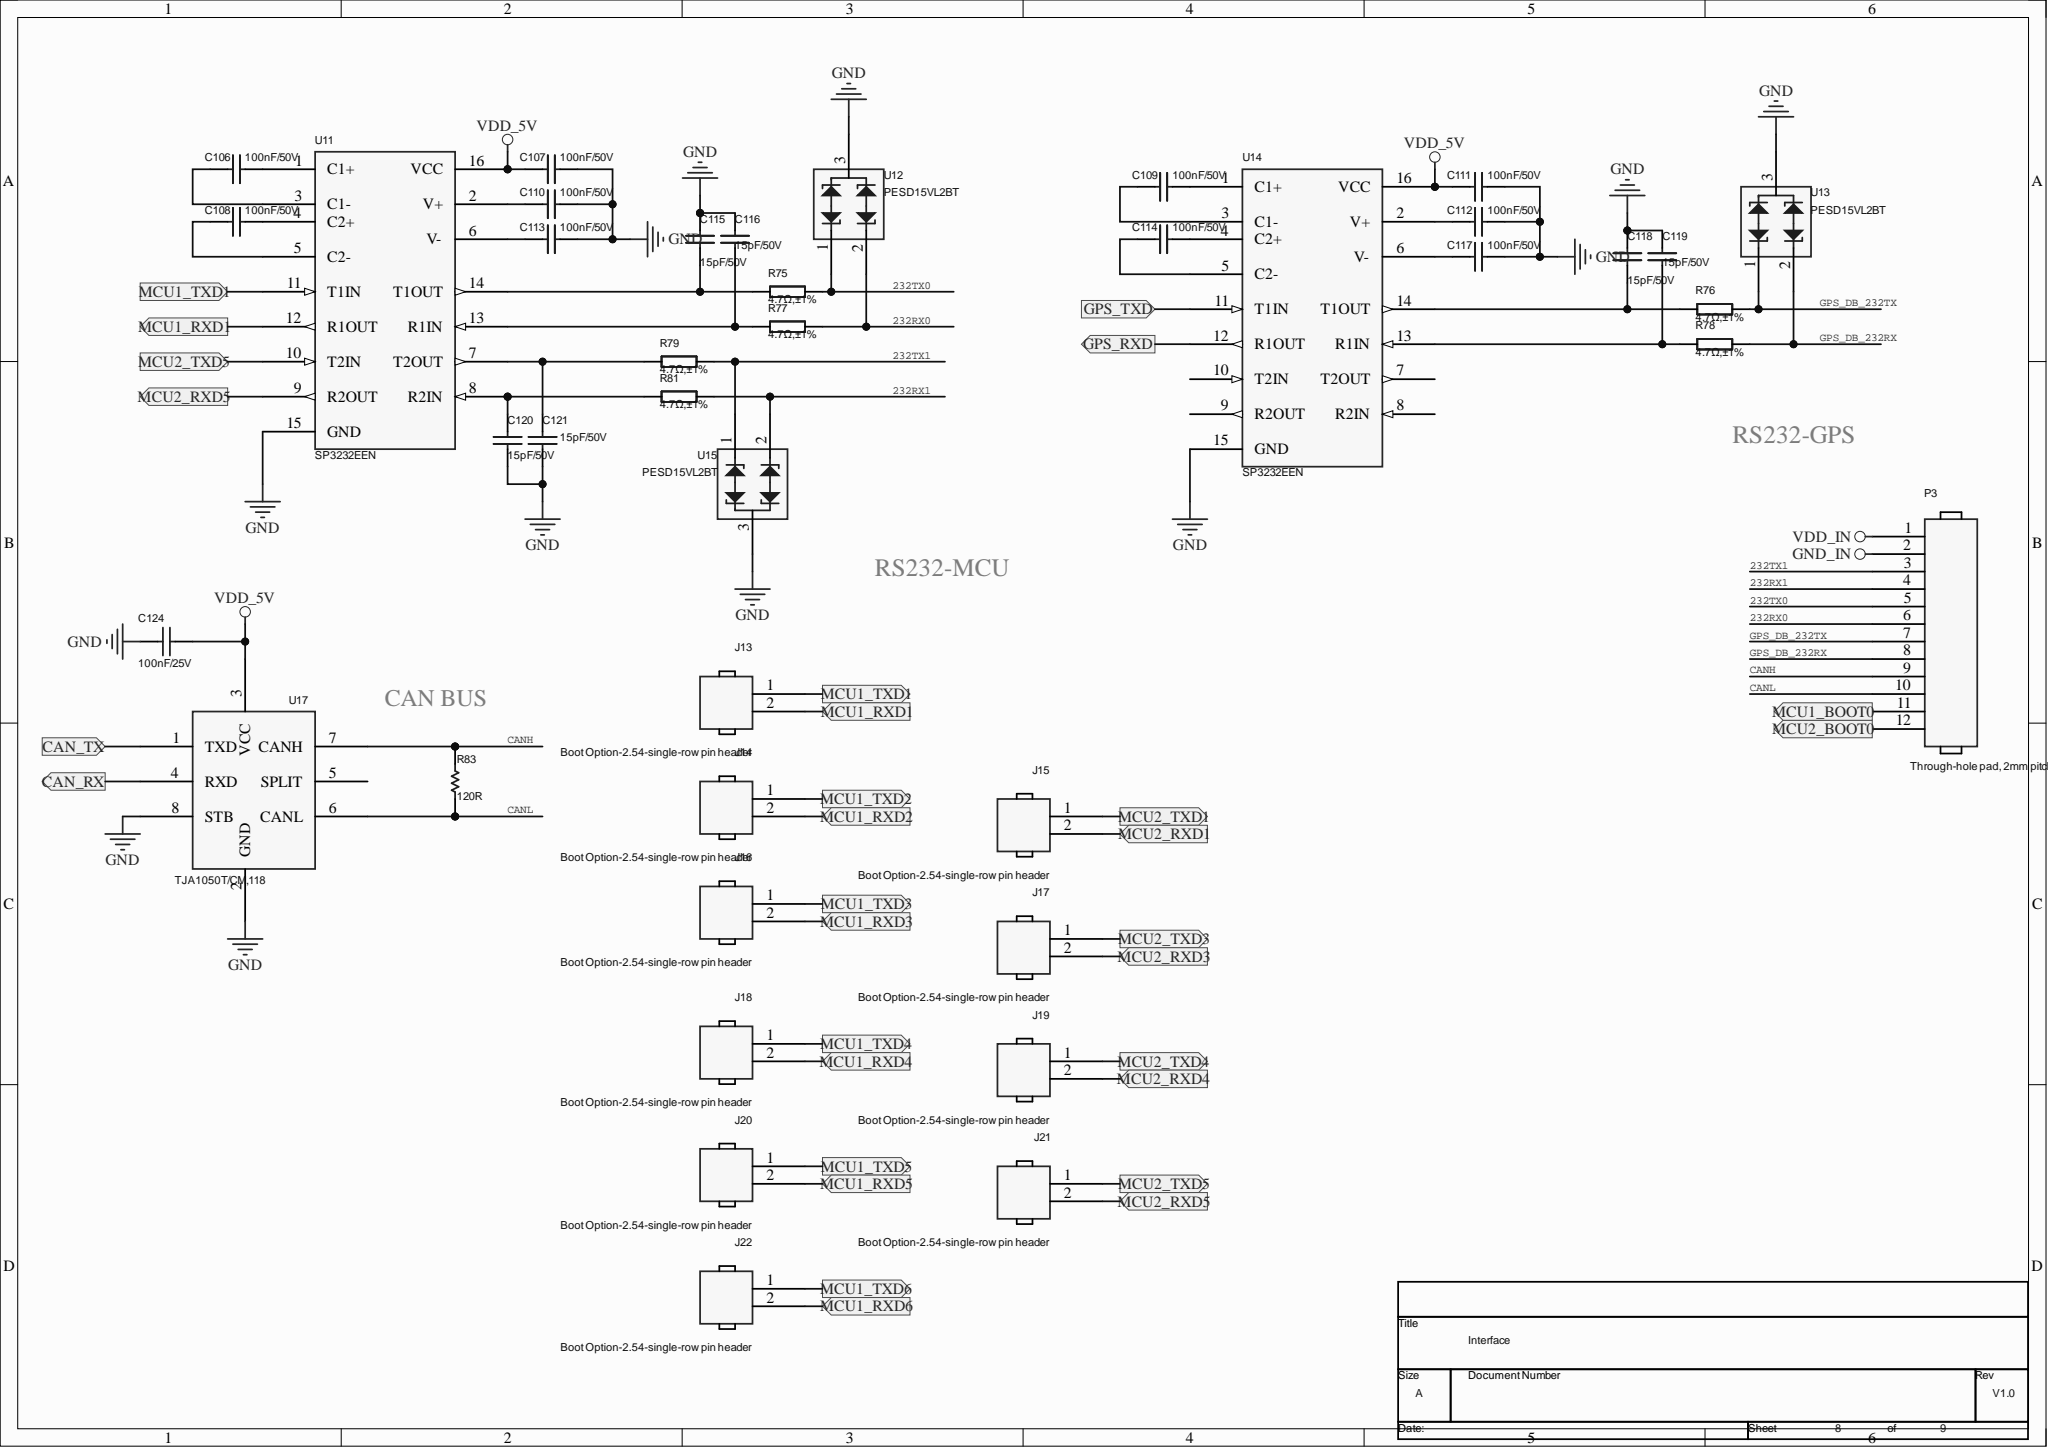Circuit board | Altium Designer | 313 parts | 216 nets | one sheet of the schematic
Parts on this sheet (reference | value | footprint):
C106 | 100nF/50V | 0603
C107 | 100nF/50V | 0603
C108 | 100nF/50V | 0603
C109 | 100nF/50V | 0603
C110 | 100nF/50V | 0603
C111 | 100nF/50V | 0603
C112 | 100nF/50V | 0603
C113 | 100nF/50V | 0603
C114 | 100nF/50V | 0603
C115 | 15pF/50V | 0603
C116 | 15pF/50V | 0603
C117 | 100nF/50V | 0603
C118 | 15pF/50V | 0603
C119 | 15pF/50V | 0603
C120 | 15pF/50V | 0603
C121 | 15pF/50V | 0603
C124 | 100nF/50V | C0603
J13 | Boot Option-2.54-single-row pin header | HDR_1X2_254
J14 | Boot Option-2.54-single-row pin header | HDR_1X2_254
J15 | Boot Option-2.54-single-row pin header | HDR_1X2_254
J16 | Boot Option-2.54-single-row pin header | HDR_1X2_254
J17 | Boot Option-2.54-single-row pin header | HDR_1X2_254
J18 | Boot Option-2.54-single-row pin header | HDR_1X2_254
J19 | Boot Option-2.54-single-row pin header | HDR_1X2_254
J20 | Boot Option-2.54-single-row pin header | HDR_1X2_254
J21 | Boot Option-2.54-single-row pin header | HDR_1X2_254
J22 | Boot Option-2.54-single-row pin header | HDR_1X2_254
P3 | Through-hole pad, 2mm pitch | XH-12A
R75 | 4.7Ω,±1% | 0603
R76 | 4.7Ω,±1% | 0603
R77 | 4.7Ω,±1% | 0603
R78 | 4.7Ω,±1% | 0603
R79 | 4.7Ω,±1% | 0603
R81 | 4.7Ω,±1% | 0603
R83 | 120R | R0603
U11 | SP3232EEN | SOP16-6_6
U12 | PESD15VL2BT | SOT-23
U13 | PESD15VL2BT | SOT-23
U14 | SP3232EEN | SOP16-6_6
U15 | PESD15VL2BT | SOT-23
U17 | TJA1050T/CM,118 | SOIC-8
Nets of these parts (net: part-pin ...):
VDD_IN: P3-1
VDD_5V: C107-1 C111-1 C124-2 U11-16 U14-16 U17-3
NetU1_104: U17-1
NetU1_103: U17-4
NetP3_12: P3-12
NetP3_11: P3-11
NetJ22_2: J22-2
NetJ22_1: J22-1
NetJ21_2: J21-2 U11-9
NetJ21_1: J21-1 U11-10
NetJ19_2: J19-2
NetJ19_1: J19-1
NetJ17_2: J17-2
NetJ17_1: J17-1
NetJ16_2: J16-2
NetJ16_1: J16-1
NetJ14_2: J14-2
NetJ14_1: J14-1
NetJ13_2: J13-2 U11-12
NetJ13_1: J13-1 U11-11
NetJ6_40: J20-1
NetJ6_39: J20-2
NetJ6_38: J15-1
NetJ6_37: J15-2
NetJ6_36: U14-12
NetJ6_35: U14-11
NetC121_1: C121-1 R79-2 U11-7
NetC120_1: C120-1 R81-2 U11-8
NetC119_2: C119-2 R78-2 U14-13
NetC118_2: C118-2 R76-2 U14-14
NetC117_1: C117-1 U14-6
NetC116_2: C116-2 R77-2 U11-13
NetC115_2: C115-2 R75-2 U11-14
NetC114_2: C114-2 U14-4
NetC114_1: C114-1 U14-5
NetC113_1: C113-1 U11-6
NetC112_1: C112-1 U14-2
NetC110_1: C110-1 U11-2
NetC109_2: C109-2 U14-1
NetC109_1: C109-1 U14-3
NetC108_2: C108-2 U11-4
NetC108_1: C108-1 U11-5
NetC106_2: C106-2 U11-1
NetC106_1: C106-1 U11-3
IMU_TXD1: J18-2
IMU_RXD1: J18-1
GPS_DB_232TX: P3-7 R76-1 U13-1
GPS_DB_232RX: P3-8 R78-1 U13-2
GND_IN: P3-2
GND: C107-2 C110-2 C111-2 C112-2 C113-2 C115-1 C116-1 C117-2 C118-1 C119-1 C120-2 C121-2 C124-1 U11-15 U12-3 U13-3 U14-15 U15-3 U17-2 U17-8
CANL: P3-10 R83-2 U17-6
CANH: P3-9 R83-1 U17-7
232TX1: P3-3 R79-1 U15-1
232TX0: P3-5 R75-1 U12-1
232RX1: P3-4 R81-1 U15-2
232RX0: P3-6 R77-1 U12-2